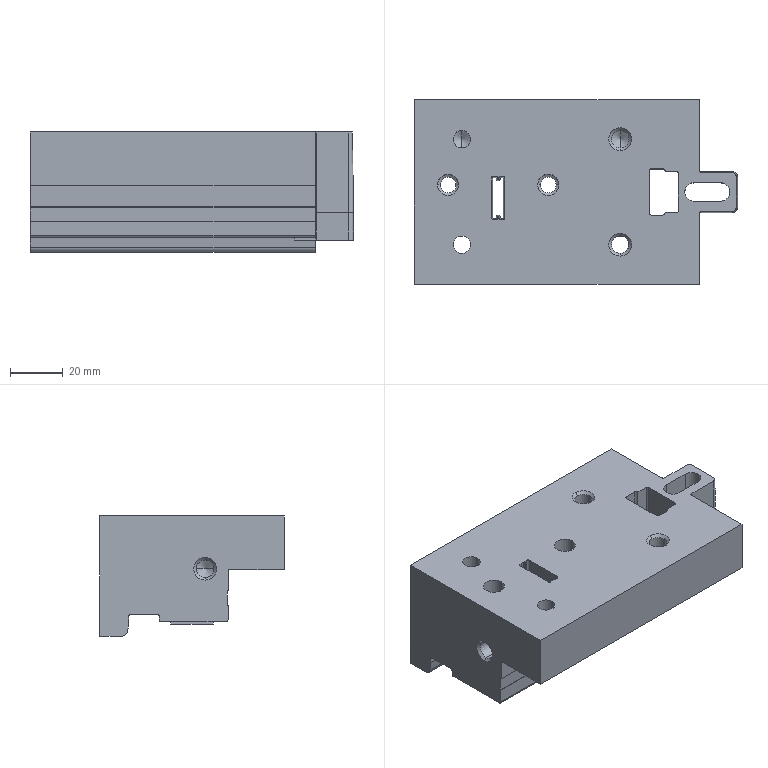Part | STEP file | KHUON AM_2 | 1 solid | 133 faces | box 122.5 x 70 x 45.5 mm | volume 246860 mm3 | plane 58 | cylinder 47 | cone 28 | commonest cylinder face diameters 6.647 x10 1.6 x6 0.2 x4 0.4 x4 1 x4 6 x4